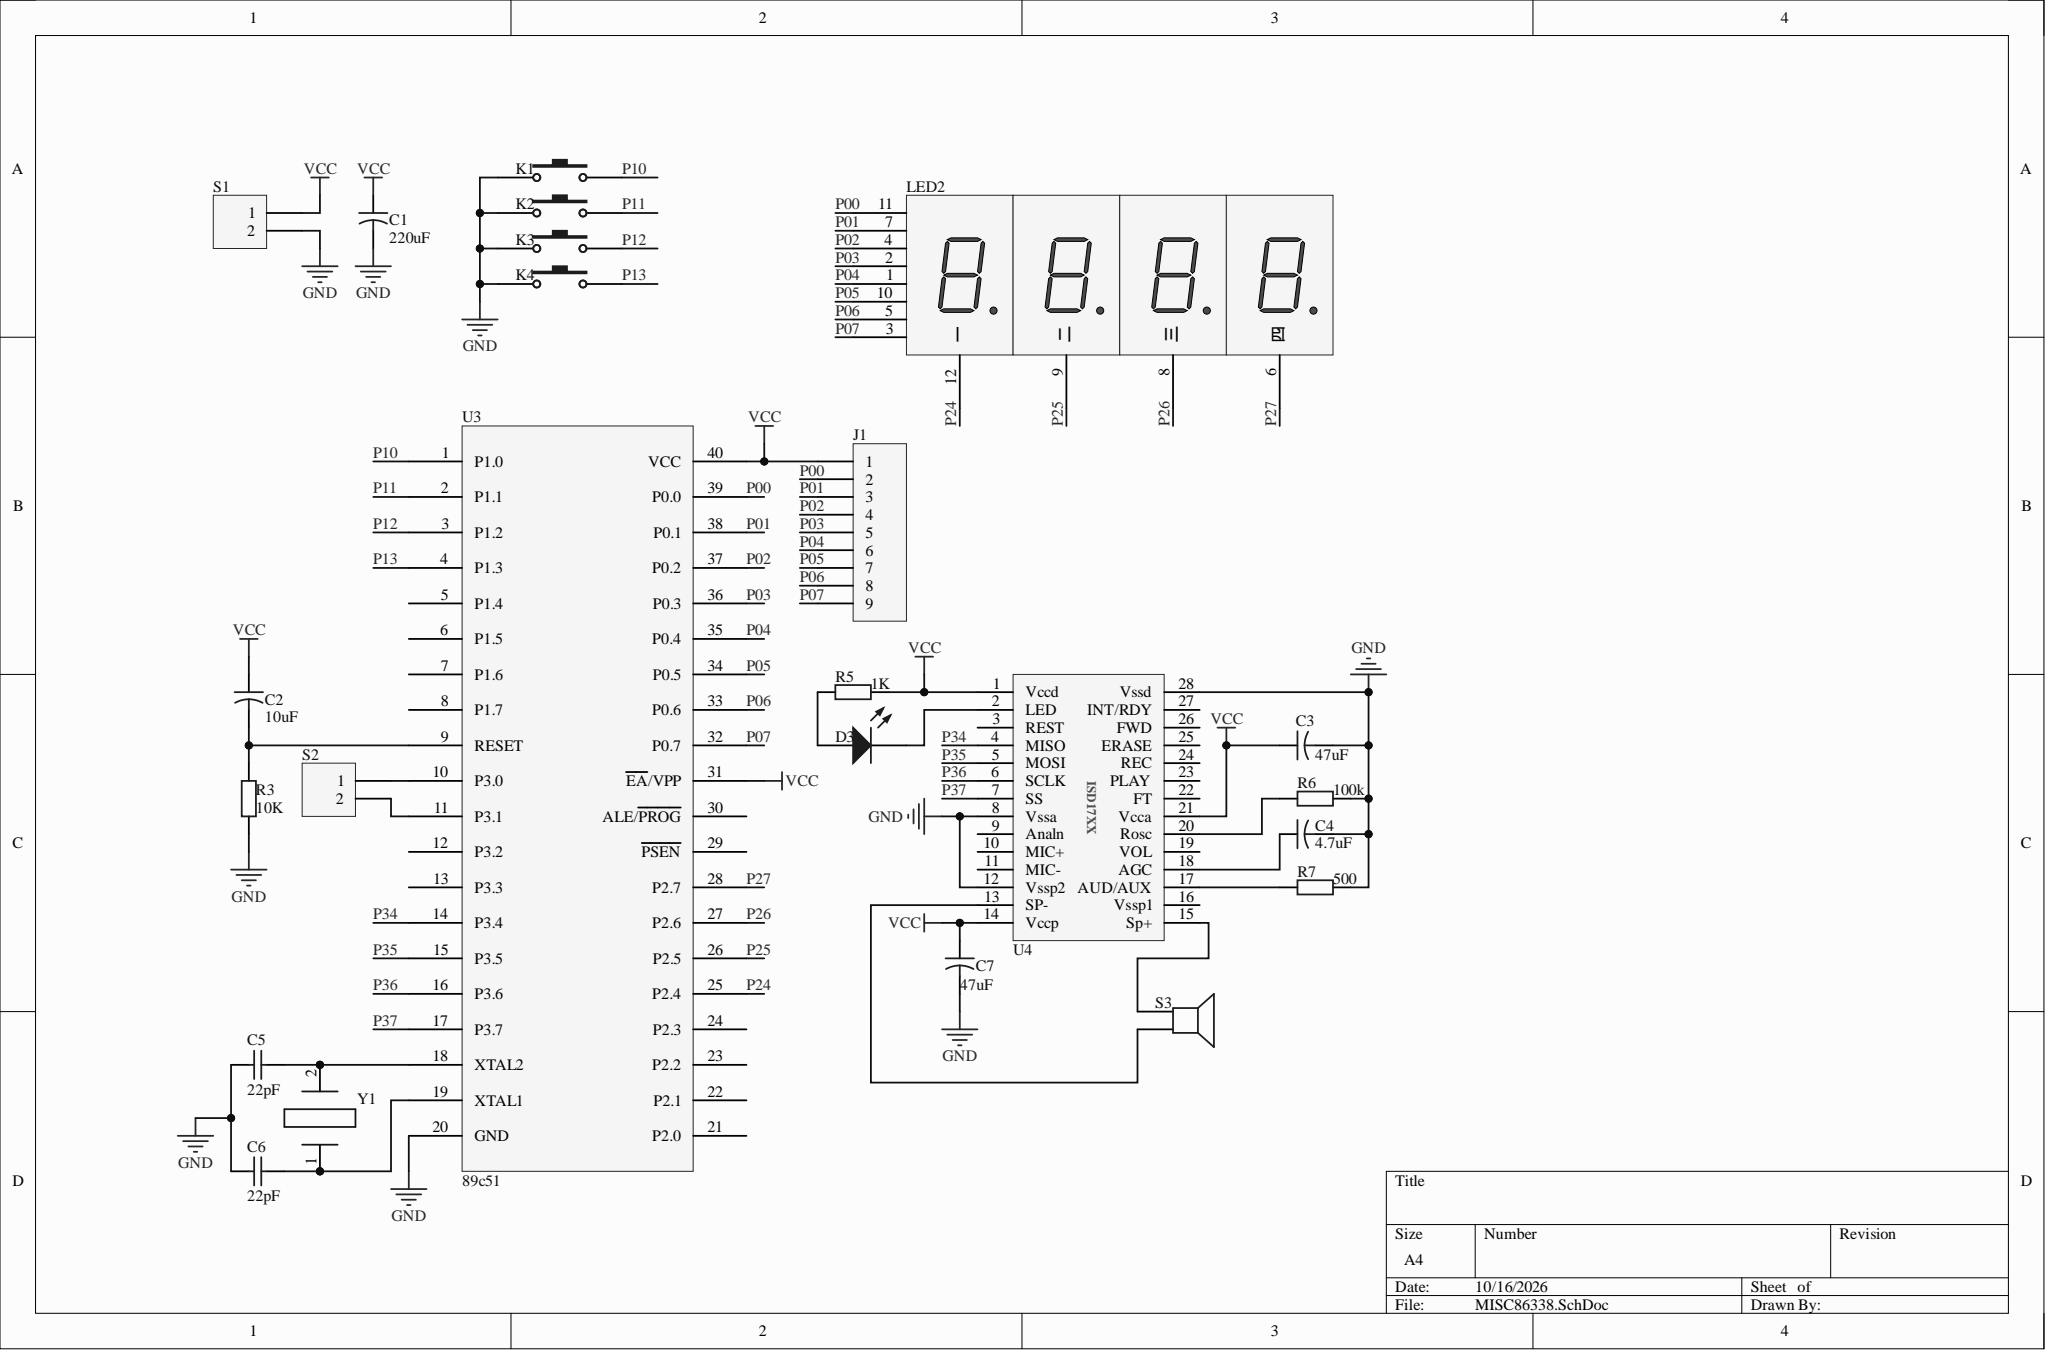Circuit board | Altium Designer | 24 parts | 34 nets
Bill of materials:
Comment,Description,Designator,Footprint,LibRef,Quantity
"Cap2","Capacitor","C1, C2, C3, C4, C7","CAPR5-4X5","Cap2","5"
"Cap","Capacitor","C5, C6","RAD-0.3","Cap","2"
"LED1","Typical RED GaAs LED","D3","LED-1","LED1","1"
"Header 9","Header, 9-Pin","J1","HDR1X9","Header 9","1"
"SW-PB","Switch","K1, K2, K3, K4","SPST-2","SW-PB","4"
"Dpy Red-CA","7.62 mm Black Surface HER 7-Segment Display: CA, RH DP","LED2","四位数码管","Dpy Red-CA","1"
"Res2","Resistor","R3, R5, R6, R7","AXIAL-0.4","Res2","4"
"Header 2","Header, 2-Pin","S1, S2","HDR1X2","Header 2","2"
"Speaker","Loudspeaker","S3","PIN2","Speaker","1"
"89c51","","U3","89c51","Component_1","1"
"Component_1","","U4","ISD1730","Component_1","1"
"Component_1","","Y1","XTAL","Component_1","1"
Netlist (Protel format):
[
C1
CAPR5-4X5
Cap2



]
[
C2
CAPR5-4X5
Cap2



]
[
C3
CAPR5-4X5
Cap2



]
[
C4
CAPR5-4X5
Cap2



]
[
C5
RAD-0.3
Cap



]
[
C6
RAD-0.3
Cap



]
[
C7
CAPR5-4X5
Cap2



]
[
D3
LED-1
LED1



]
[
J1
HDR1X9
Header 9



]
[
K1
SPST-2
SW-PB



]
[
K2
SPST-2
SW-PB



]
[
K3
SPST-2
SW-PB



]
[
K4
SPST-2
SW-PB



]
[
LED2
四位数码管
Dpy Red-CA



]
[
R3
AXIAL-0.4
Res2



]
[
R5
AXIAL-0.4
Res2



]
[
R6
AXIAL-0.4
Res2



]
[
R7
AXIAL-0.4
Res2



]
[
S1
HDR1X2
Header 2



]
[
S2
HDR1X2
Header 2



]
[
S3
PIN2
Speaker



]
[
U3
89c51
89c51



]
[
U4
ISD1730
Component_1



]
[
Y1
XTAL
Component_1



]
(
VCC
C1-1
C2-1
C3-1
C7-1
J1-1
R5-1
S1-1
U3-31
U3-40
U4-1
U4-14
U4-21
)
(
P37
U3-17
U4-7
)
(
P36
U3-16
U4-6
)
(
P35
U3-15
U4-5
)
(
P34
U3-14
U4-4
)
(
P27
LED2-6
U3-28
)
(
P26
LED2-8
U3-27
)
(
P25
LED2-9
U3-26
)
(
P24
LED2-12
U3-25
)
(
P13
K4-2
U3-4
)
(
P12
K3-2
U3-3
)
(
P11
K2-2
U3-2
)
(
P10
K1-2
U3-1
)
(
P07
J1-9
LED2-3
U3-32
)
(
P06
J1-8
LED2-5
U3-33
)
(
P05
J1-7
LED2-10
U3-34
)
(
P04
J1-6
LED2-1
U3-35
)
(
P03
J1-5
LED2-2
U3-36
)
(
P02
J1-4
LED2-4
U3-37
)
(
P01
J1-3
LED2-7
U3-38
)
(
P00
J1-2
LED2-11
U3-39
)
(
NetS3_2
S3-2
U4-13
)
(
NetS3_1
S3-1
U4-15
)
(
NetS2_2
S2-2
U3-11
)
(
NetS2_1
S2-1
U3-10
)
(
NetR7_2
R7-2
U4-17
)
(
NetR6_2
R6-2
U4-20
)
(
NetD3_2
D3-2
U4-2
)
(
NetD3_1
D3-1
R5-2
)
(
NetC6_2
C6-2
U3-19
Y1-1
)
(
NetC5_2
C5-2
U3-18
Y1-2
)
(
NetC4_1
C4-1
U4-18
)
(
NetC2_2
C2-2
R3-2
U3-9
)
(
GND
C1-2
C3-2
C4-2
C5-1
C6-1
C7-2
K1-1
K2-1
K3-1
K4-1
R3-1
R6-1
R7-1
S1-2
U3-20
U4-8
U4-12
U4-28
)